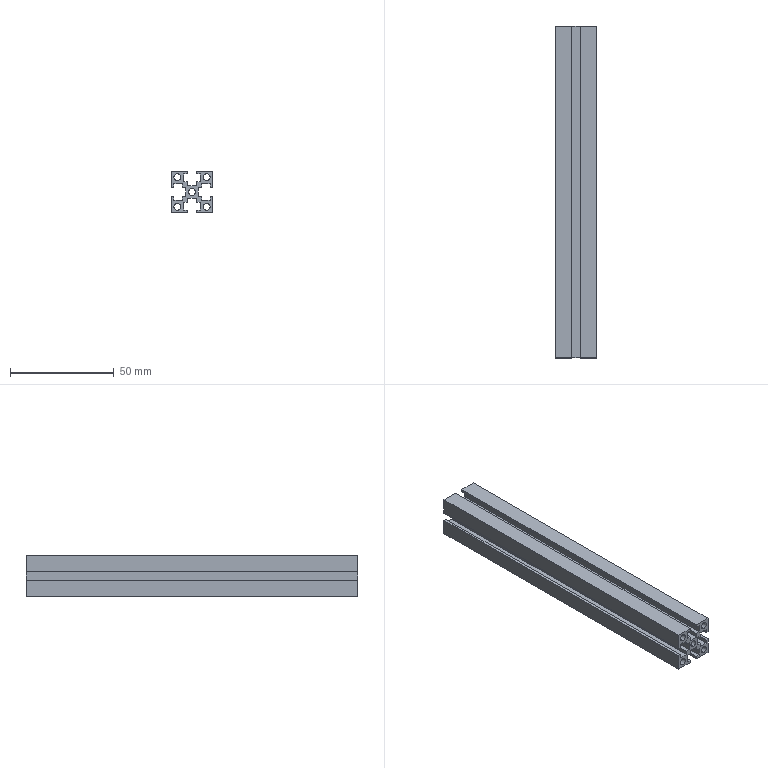Part | STEP file | 20 aluminium profile diagonal 2 | 1 solid | 64 faces | box 20 x 160 x 20 mm | volume 28445 mm3 | plane 54 | cylinder 10 | commonest cylinder face diameters 3.3 x10